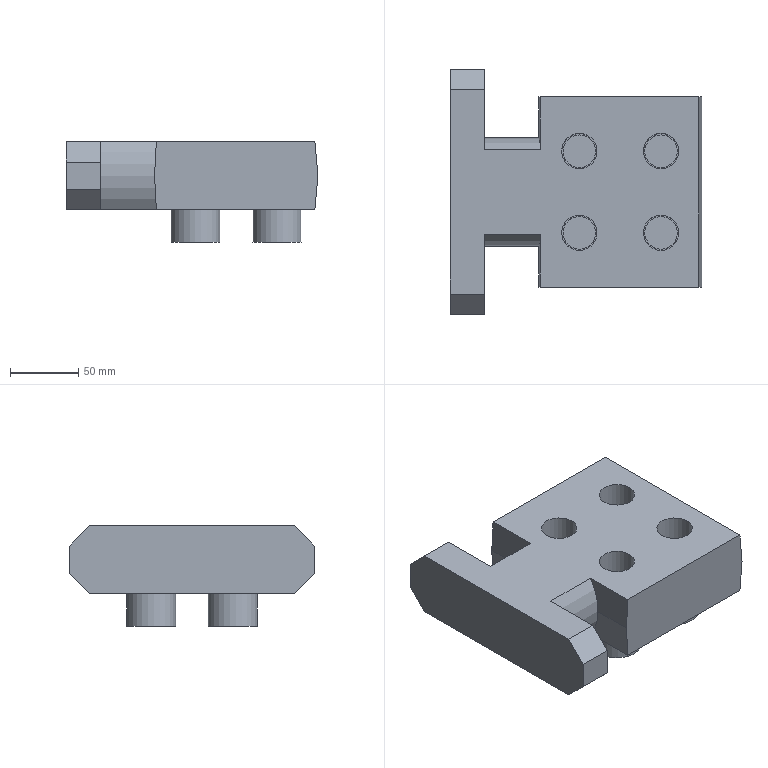Part | STEP file | MI_CHPL_0008_id2058_x_t | 1 solid | 149 faces | box 185 x 180 x 74 mm | volume 1174333 mm3 | plane 113 | cylinder 36 | commonest cylinder face diameters 24 x4 26 x4 36 x4 6.746 x2 8.429 x2 80 x2